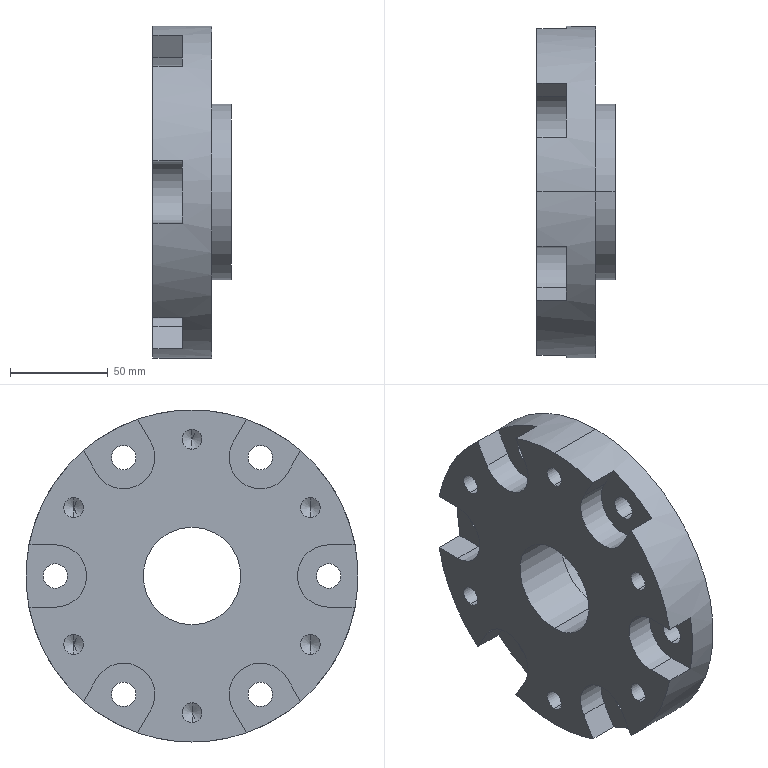Part | SolidWorks | features CirPattern 3, ICE 3, 3DProfileFeature 1, HoleWzd 1, Revolution 1 | 1 solid | 74 faces | box 40 x 170 x 170 mm | volume 559070 mm3 | cylinder 40 | plane 22 | cone 12 | commonest cylinder face diameters 10.2 x12 12.5 x12 32 x8 50 x2 60 x2 90 x2